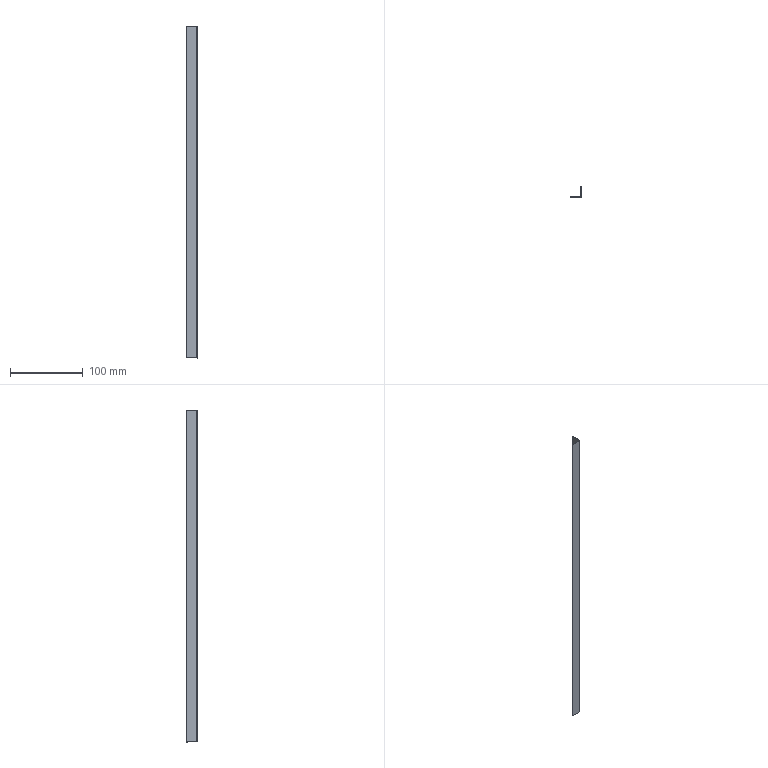Part | SolidWorks | features SplitBody 1 | 1 solid | 14 faces | box 15 x 15 x 456 mm | volume 13107 mm3 | plane 12 | cylinder 2 | commonest cylinder face diameters 0.2 x1 2.2 x1
STEP:
#1=CARTESIAN_POINT('',(547.9,781.75,208.));
#2=VERTEX_POINT('',#1);
#3=CARTESIAN_POINT('',(547.9,782.75,208.));
#4=VERTEX_POINT('',#3);
#5=CARTESIAN_POINT('',(547.9,781.75,208.));
#6=DIRECTION('',(0.,1.,0.));
#7=VECTOR('',#6,1000.);
#8=LINE('',#5,#7);
#9=EDGE_CURVE('',#2,#4,#8,.T.);
#10=ORIENTED_EDGE('',*,*,#9,.F.);
#11=CARTESIAN_POINT('',(549.,782.85,208.));
#12=VERTEX_POINT('',#11);
#13=CARTESIAN_POINT('',(547.9,782.85,208.));
#14=DIRECTION('',(0.,0.,1.));
#15=DIRECTION('',(-1.,0.,0.));
#16=AXIS2_PLACEMENT_3D('',#13,#14,#15);
#17=CIRCLE('',#16,1.1);
#18=EDGE_CURVE('',#2,#12,#17,.T.);
#19=ORIENTED_EDGE('',*,*,#18,.T.);
#20=CARTESIAN_POINT('',(548.,782.85,208.));
#21=VERTEX_POINT('',#20);
#22=CARTESIAN_POINT('',(548.,782.85,208.));
#23=DIRECTION('',(1.,0.,0.));
#24=VECTOR('',#23,1000.);
#25=LINE('',#22,#24);
#26=EDGE_CURVE('',#21,#12,#25,.T.);
#27=ORIENTED_EDGE('',*,*,#26,.F.);
#28=CARTESIAN_POINT('',(547.9,782.85,208.));
#29=DIRECTION('',(0.,0.,1.));
#30=DIRECTION('',(-1.,0.,0.));
#31=AXIS2_PLACEMENT_3D('',#28,#29,#30);
#32=CIRCLE('',#31,0.1);
#33=EDGE_CURVE('',#4,#21,#32,.T.);
#34=ORIENTED_EDGE('',*,*,#33,.F.);
#35=EDGE_LOOP('',(#10,#19,#27,#34));
#36=FACE_OUTER_BOUND('',#35,.T.);
#37=CARTESIAN_POINT('',(547.9,781.75,208.));
#38=DIRECTION('',(0.,0.,1.));
#39=DIRECTION('',(1.,0.,0.));
#40=AXIS2_PLACEMENT_3D('',#37,#38,#39);
#41=PLANE('',#40);
#42=ADVANCED_FACE('',(#36),#41,.T.);
#43=CARTESIAN_POINT('',(534.,781.75,208.));
#44=VERTEX_POINT('',#43);
#45=CARTESIAN_POINT('',(549.,781.75,208.));
#46=DIRECTION('',(1.,0.,0.));
#47=VECTOR('',#46,1000.);
#48=LINE('',#45,#47);
#49=EDGE_CURVE('',#44,#2,#48,.T.);
#50=ORIENTED_EDGE('',*,*,#49,.T.);
#51=ORIENTED_EDGE('',*,*,#9,.T.);
#52=CARTESIAN_POINT('',(534.,782.75,208.));
#53=VERTEX_POINT('',#52);
#54=CARTESIAN_POINT('',(549.,782.75,208.));
#55=DIRECTION('',(1.,0.,0.));
#56=VECTOR('',#55,1000.);
#57=LINE('',#54,#56);
#58=EDGE_CURVE('',#53,#4,#57,.T.);
#59=ORIENTED_EDGE('',*,*,#58,.F.);
#60=CARTESIAN_POINT('',(534.,782.75,208.));
#61=DIRECTION('',(0.,-1.,0.));
#62=VECTOR('',#61,1000.);
#63=LINE('',#60,#62);
#64=EDGE_CURVE('',#53,#44,#63,.T.);
#65=ORIENTED_EDGE('',*,*,#64,.T.);
#66=EDGE_LOOP('',(#50,#51,#59,#65));
#67=FACE_OUTER_BOUND('',#66,.T.);
#68=CARTESIAN_POINT('',(548.,782.85,208.));
#69=DIRECTION('',(0.,0.,1.));
#70=DIRECTION('',(1.,0.,0.));
#71=AXIS2_PLACEMENT_3D('',#68,#69,#70);
#72=PLANE('',#71);
#73=ADVANCED_FACE('',(#67),#72,.T.);
#74=CARTESIAN_POINT('',(548.,796.75,-248.));
#75=VERTEX_POINT('',#74);
#76=CARTESIAN_POINT('',(548.,782.85,-248.));
#77=VERTEX_POINT('',#76);
#78=CARTESIAN_POINT('',(548.,781.75,-248.));
#79=DIRECTION('',(0.,-1.,0.));
#80=VECTOR('',#79,1000.);
#81=LINE('',#78,#80);
#82=EDGE_CURVE('',#75,#77,#81,.T.);
#83=ORIENTED_EDGE('',*,*,#82,.T.);
#84=CARTESIAN_POINT('',(548.,782.85,-269.213));
#85=DIRECTION('',(0.,0.,1.));
#86=VECTOR('',#85,1000.);
#87=LINE('',#84,#86);
#88=EDGE_CURVE('',#77,#21,#87,.T.);
#89=ORIENTED_EDGE('',*,*,#88,.T.);
#90=CARTESIAN_POINT('',(548.,796.75,208.));
#91=VERTEX_POINT('',#90);
#92=CARTESIAN_POINT('',(548.,781.75,208.));
#93=DIRECTION('',(0.,1.,0.));
#94=VECTOR('',#93,1000.);
#95=LINE('',#92,#94);
#96=EDGE_CURVE('',#21,#91,#95,.T.);
#97=ORIENTED_EDGE('',*,*,#96,.T.);
#98=CARTESIAN_POINT('',(548.,796.75,-269.213));
#99=DIRECTION('',(0.,0.,1.));
#100=VECTOR('',#99,1000.);
#101=LINE('',#98,#100);
#102=EDGE_CURVE('',#75,#91,#101,.T.);
#103=ORIENTED_EDGE('',*,*,#102,.F.);
#104=EDGE_LOOP('',(#83,#89,#97,#103));
#105=FACE_OUTER_BOUND('',#104,.T.);
#106=CARTESIAN_POINT('',(548.,781.75,-269.213));
#107=DIRECTION('',(1.,0.,0.));
#108=DIRECTION('',(0.,0.,-1.));
#109=AXIS2_PLACEMENT_3D('',#106,#107,#108);
#110=PLANE('',#109);
#111=ADVANCED_FACE('',(#105),#110,.F.);
#112=CARTESIAN_POINT('',(549.,796.75,-248.));
#113=VERTEX_POINT('',#112);
#114=CARTESIAN_POINT('',(549.,796.75,208.));
#115=VERTEX_POINT('',#114);
#116=CARTESIAN_POINT('',(549.,796.75,-269.213));
#117=DIRECTION('',(0.,0.,1.));
#118=VECTOR('',#117,1000.);
#119=LINE('',#116,#118);
#120=EDGE_CURVE('',#113,#115,#119,.T.);
#121=ORIENTED_EDGE('',*,*,#120,.F.);
#122=CARTESIAN_POINT('',(548.,796.75,-248.));
#123=DIRECTION('',(1.,0.,0.));
#124=VECTOR('',#123,1000.);
#125=LINE('',#122,#124);
#126=EDGE_CURVE('',#75,#113,#125,.T.);
#127=ORIENTED_EDGE('',*,*,#126,.F.);
#128=ORIENTED_EDGE('',*,*,#102,.T.);
#129=CARTESIAN_POINT('',(549.,796.75,208.));
#130=DIRECTION('',(-1.,0.,0.));
#131=VECTOR('',#130,1000.);
#132=LINE('',#129,#131);
#133=EDGE_CURVE('',#115,#91,#132,.T.);
#134=ORIENTED_EDGE('',*,*,#133,.F.);
#135=EDGE_LOOP('',(#121,#127,#128,#134));
#136=FACE_OUTER_BOUND('',#135,.T.);
#137=CARTESIAN_POINT('',(549.,796.75,-269.213));
#138=DIRECTION('',(0.,1.,0.));
#139=DIRECTION('',(0.,0.,1.));
#140=AXIS2_PLACEMENT_3D('',#137,#138,#139);
#141=PLANE('',#140);
#142=ADVANCED_FACE('',(#136),#141,.T.);
#143=CARTESIAN_POINT('',(549.,782.85,-248.));
#144=VERTEX_POINT('',#143);
#145=CARTESIAN_POINT('',(549.,782.85,-269.213));
#146=DIRECTION('',(0.,0.,1.));
#147=VECTOR('',#146,1000.);
#148=LINE('',#145,#147);
#149=EDGE_CURVE('',#144,#12,#148,.T.);
#150=ORIENTED_EDGE('',*,*,#149,.F.);
#151=CARTESIAN_POINT('',(549.,781.75,-248.));
#152=DIRECTION('',(0.,-1.,0.));
#153=VECTOR('',#152,1000.);
#154=LINE('',#151,#153);
#155=EDGE_CURVE('',#113,#144,#154,.T.);
#156=ORIENTED_EDGE('',*,*,#155,.F.);
#157=ORIENTED_EDGE('',*,*,#120,.T.);
#158=CARTESIAN_POINT('',(549.,781.75,208.));
#159=DIRECTION('',(0.,1.,0.));
#160=VECTOR('',#159,1000.);
#161=LINE('',#158,#160);
#162=EDGE_CURVE('',#12,#115,#161,.T.);
#163=ORIENTED_EDGE('',*,*,#162,.F.);
#164=EDGE_LOOP('',(#150,#156,#157,#163));
#165=FACE_OUTER_BOUND('',#164,.T.);
#166=CARTESIAN_POINT('',(549.,781.75,-269.213));
#167=DIRECTION('',(1.,0.,0.));
#168=DIRECTION('',(0.,0.,-1.));
#169=AXIS2_PLACEMENT_3D('',#166,#167,#168);
#170=PLANE('',#169);
#171=ADVANCED_FACE('',(#165),#170,.T.);
#172=CARTESIAN_POINT('',(547.9,781.75,-248.));
#173=VERTEX_POINT('',#172);
#174=CARTESIAN_POINT('',(547.9,781.75,-269.213));
#175=DIRECTION('',(0.,0.,1.));
#176=VECTOR('',#175,1000.);
#177=LINE('',#174,#176);
#178=EDGE_CURVE('',#173,#2,#177,.T.);
#179=ORIENTED_EDGE('',*,*,#178,.F.);
#180=CARTESIAN_POINT('',(547.9,782.85,-248.));
#181=DIRECTION('',(0.,0.,-1.));
#182=DIRECTION('',(-1.,0.,0.));
#183=AXIS2_PLACEMENT_3D('',#180,#181,#182);
#184=CIRCLE('',#183,1.1);
#185=EDGE_CURVE('',#144,#173,#184,.T.);
#186=ORIENTED_EDGE('',*,*,#185,.F.);
#187=ORIENTED_EDGE('',*,*,#149,.T.);
#188=ORIENTED_EDGE('',*,*,#18,.F.);
#189=EDGE_LOOP('',(#179,#186,#187,#188));
#190=FACE_OUTER_BOUND('',#189,.T.);
#191=CARTESIAN_POINT('',(547.9,782.85,-269.213));
#192=DIRECTION('',(0.,0.,1.));
#193=DIRECTION('',(1.,0.,0.));
#194=AXIS2_PLACEMENT_3D('',#191,#192,#193);
#195=CYLINDRICAL_SURFACE('',#194,1.1);
#196=ADVANCED_FACE('',(#190),#195,.T.);
#197=CARTESIAN_POINT('',(534.,781.75,-248.));
#198=VERTEX_POINT('',#197);
#199=CARTESIAN_POINT('',(534.,781.75,-269.213));
#200=DIRECTION('',(0.,0.,1.));
#201=VECTOR('',#200,1000.);
#202=LINE('',#199,#201);
#203=EDGE_CURVE('',#198,#44,#202,.T.);
#204=ORIENTED_EDGE('',*,*,#203,.F.);
#205=CARTESIAN_POINT('',(549.,781.75,-248.));
#206=DIRECTION('',(-1.,0.,0.));
#207=VECTOR('',#206,1000.);
#208=LINE('',#205,#207);
#209=EDGE_CURVE('',#173,#198,#208,.T.);
#210=ORIENTED_EDGE('',*,*,#209,.F.);
#211=ORIENTED_EDGE('',*,*,#178,.T.);
#212=ORIENTED_EDGE('',*,*,#49,.F.);
#213=EDGE_LOOP('',(#204,#210,#211,#212));
#214=FACE_OUTER_BOUND('',#213,.T.);
#215=CARTESIAN_POINT('',(549.,781.75,-269.213));
#216=DIRECTION('',(0.,-1.,0.));
#217=DIRECTION('',(0.,0.,-1.));
#218=AXIS2_PLACEMENT_3D('',#215,#216,#217);
#219=PLANE('',#218);
#220=ADVANCED_FACE('',(#214),#219,.T.);
#221=CARTESIAN_POINT('',(534.,782.75,-248.));
#222=VERTEX_POINT('',#221);
#223=CARTESIAN_POINT('',(534.,782.75,-269.213));
#224=DIRECTION('',(0.,0.,1.));
#225=VECTOR('',#224,1000.);
#226=LINE('',#223,#225);
#227=EDGE_CURVE('',#222,#53,#226,.T.);
#228=ORIENTED_EDGE('',*,*,#227,.F.);
#229=CARTESIAN_POINT('',(534.,782.75,-248.));
#230=DIRECTION('',(0.,-1.,0.));
#231=VECTOR('',#230,1000.);
#232=LINE('',#229,#231);
#233=EDGE_CURVE('',#222,#198,#232,.T.);
#234=ORIENTED_EDGE('',*,*,#233,.T.);
#235=ORIENTED_EDGE('',*,*,#203,.T.);
#236=ORIENTED_EDGE('',*,*,#64,.F.);
#237=EDGE_LOOP('',(#228,#234,#235,#236));
#238=FACE_OUTER_BOUND('',#237,.T.);
#239=CARTESIAN_POINT('',(534.,782.75,-269.213));
#240=DIRECTION('',(-1.,0.,0.));
#241=DIRECTION('',(0.,0.,1.));
#242=AXIS2_PLACEMENT_3D('',#239,#240,#241);
#243=PLANE('',#242);
#244=ADVANCED_FACE('',(#238),#243,.T.);
#245=CARTESIAN_POINT('',(547.9,782.75,-248.));
#246=VERTEX_POINT('',#245);
#247=CARTESIAN_POINT('',(549.,782.75,-248.));
#248=DIRECTION('',(-1.,0.,0.));
#249=VECTOR('',#248,1000.);
#250=LINE('',#247,#249);
#251=EDGE_CURVE('',#246,#222,#250,.T.);
#252=ORIENTED_EDGE('',*,*,#251,.T.);
#253=ORIENTED_EDGE('',*,*,#227,.T.);
#254=ORIENTED_EDGE('',*,*,#58,.T.);
#255=CARTESIAN_POINT('',(547.9,782.75,-269.213));
#256=DIRECTION('',(0.,0.,1.));
#257=VECTOR('',#256,1000.);
#258=LINE('',#255,#257);
#259=EDGE_CURVE('',#246,#4,#258,.T.);
#260=ORIENTED_EDGE('',*,*,#259,.F.);
#261=EDGE_LOOP('',(#252,#253,#254,#260));
#262=FACE_OUTER_BOUND('',#261,.T.);
#263=CARTESIAN_POINT('',(549.,782.75,-269.213));
#264=DIRECTION('',(0.,-1.,0.));
#265=DIRECTION('',(0.,0.,-1.));
#266=AXIS2_PLACEMENT_3D('',#263,#264,#265);
#267=PLANE('',#266);
#268=ADVANCED_FACE('',(#262),#267,.F.);
#269=CARTESIAN_POINT('',(547.9,782.85,-248.));
#270=DIRECTION('',(0.,0.,-1.));
#271=DIRECTION('',(1.,0.,0.));
#272=AXIS2_PLACEMENT_3D('',#269,#270,#271);
#273=CIRCLE('',#272,0.1);
#274=EDGE_CURVE('',#77,#246,#273,.T.);
#275=ORIENTED_EDGE('',*,*,#274,.T.);
#276=ORIENTED_EDGE('',*,*,#259,.T.);
#277=ORIENTED_EDGE('',*,*,#33,.T.);
#278=ORIENTED_EDGE('',*,*,#88,.F.);
#279=EDGE_LOOP('',(#275,#276,#277,#278));
#280=FACE_OUTER_BOUND('',#279,.T.);
#281=CARTESIAN_POINT('',(547.9,782.85,-269.213));
#282=DIRECTION('',(0.,0.,1.));
#283=DIRECTION('',(1.,0.,0.));
#284=AXIS2_PLACEMENT_3D('',#281,#282,#283);
#285=CYLINDRICAL_SURFACE('',#284,0.1);
#286=ADVANCED_FACE('',(#280),#285,.F.);
#287=ORIENTED_EDGE('',*,*,#96,.F.);
#288=ORIENTED_EDGE('',*,*,#26,.T.);
#289=ORIENTED_EDGE('',*,*,#162,.T.);
#290=ORIENTED_EDGE('',*,*,#133,.T.);
#291=EDGE_LOOP('',(#287,#288,#289,#290));
#292=FACE_OUTER_BOUND('',#291,.T.);
#293=CARTESIAN_POINT('',(547.9,782.85,208.));
#294=DIRECTION('',(0.,0.,-1.));
#295=DIRECTION('',(-1.,0.,0.));
#296=AXIS2_PLACEMENT_3D('',#293,#294,#295);
#297=PLANE('',#296);
#298=ADVANCED_FACE('',(#292),#297,.F.);
#299=CARTESIAN_POINT('',(548.,782.85,-248.));
#300=DIRECTION('',(1.,0.,0.));
#301=VECTOR('',#300,1000.);
#302=LINE('',#299,#301);
#303=EDGE_CURVE('',#77,#144,#302,.T.);
#304=ORIENTED_EDGE('',*,*,#303,.F.);
#305=ORIENTED_EDGE('',*,*,#82,.F.);
#306=ORIENTED_EDGE('',*,*,#126,.T.);
#307=ORIENTED_EDGE('',*,*,#155,.T.);
#308=EDGE_LOOP('',(#304,#305,#306,#307));
#309=FACE_OUTER_BOUND('',#308,.T.);
#310=CARTESIAN_POINT('',(548.,781.75,-248.));
#311=DIRECTION('',(0.,0.,1.));
#312=DIRECTION('',(0.,-1.,0.));
#313=AXIS2_PLACEMENT_3D('',#310,#311,#312);
#314=PLANE('',#313);
#315=ADVANCED_FACE('',(#309),#314,.F.);
#316=ORIENTED_EDGE('',*,*,#233,.F.);
#317=ORIENTED_EDGE('',*,*,#251,.F.);
#318=CARTESIAN_POINT('',(547.9,782.75,-248.));
#319=DIRECTION('',(0.,-1.,0.));
#320=VECTOR('',#319,1000.);
#321=LINE('',#318,#320);
#322=EDGE_CURVE('',#246,#173,#321,.T.);
#323=ORIENTED_EDGE('',*,*,#322,.T.);
#324=ORIENTED_EDGE('',*,*,#209,.T.);
#325=EDGE_LOOP('',(#316,#317,#323,#324));
#326=FACE_OUTER_BOUND('',#325,.T.);
#327=CARTESIAN_POINT('',(549.,782.75,-248.));
#328=DIRECTION('',(0.,0.,1.));
#329=DIRECTION('',(-1.,0.,0.));
#330=AXIS2_PLACEMENT_3D('',#327,#328,#329);
#331=PLANE('',#330);
#332=ADVANCED_FACE('',(#326),#331,.F.);
#333=ORIENTED_EDGE('',*,*,#185,.T.);
#334=ORIENTED_EDGE('',*,*,#322,.F.);
#335=ORIENTED_EDGE('',*,*,#274,.F.);
#336=ORIENTED_EDGE('',*,*,#303,.T.);
#337=EDGE_LOOP('',(#333,#334,#335,#336));
#338=FACE_OUTER_BOUND('',#337,.T.);
#339=CARTESIAN_POINT('',(547.9,782.85,-248.));
#340=DIRECTION('',(0.,0.,-1.));
#341=DIRECTION('',(-1.,0.,0.));
#342=AXIS2_PLACEMENT_3D('',#339,#340,#341);
#343=PLANE('',#342);
#344=ADVANCED_FACE('',(#338),#343,.T.);
#345=CLOSED_SHELL('',(#42,#73,#111,#142,#171,#196,#220,#244,#268,#286,#298,#315,#332,#344));
#346=MANIFOLD_SOLID_BREP('',#345);
#347=CARTESIAN_POINT('',(0.,0.,0.));
#348=DIRECTION('',(0.,0.,1.));
#349=DIRECTION('',(1.,0.,0.));
#350=AXIS2_PLACEMENT_3D('',#347,#348,#349);
#351=(LENGTH_UNIT()NAMED_UNIT(*)SI_UNIT(.MILLI.,.METRE.));
#352=UNCERTAINTY_MEASURE_WITH_UNIT(LENGTH_MEASURE(0.00001),#351,'','');
#353=(NAMED_UNIT(*)PLANE_ANGLE_UNIT()SI_UNIT($,.RADIAN.));
#354=(NAMED_UNIT(*)SI_UNIT($,.STERADIAN.)SOLID_ANGLE_UNIT());
#355=(GEOMETRIC_REPRESENTATION_CONTEXT(3)GLOBAL_UNCERTAINTY_ASSIGNED_CONTEXT((#352))GLOBAL_UNIT_ASSIGNED_CONTEXT((#351,#353,#354))REPRESENTATION_CONTEXT('',''));
#356=ADVANCED_BREP_SHAPE_REPRESENTATION('',(#346,#350),#355);